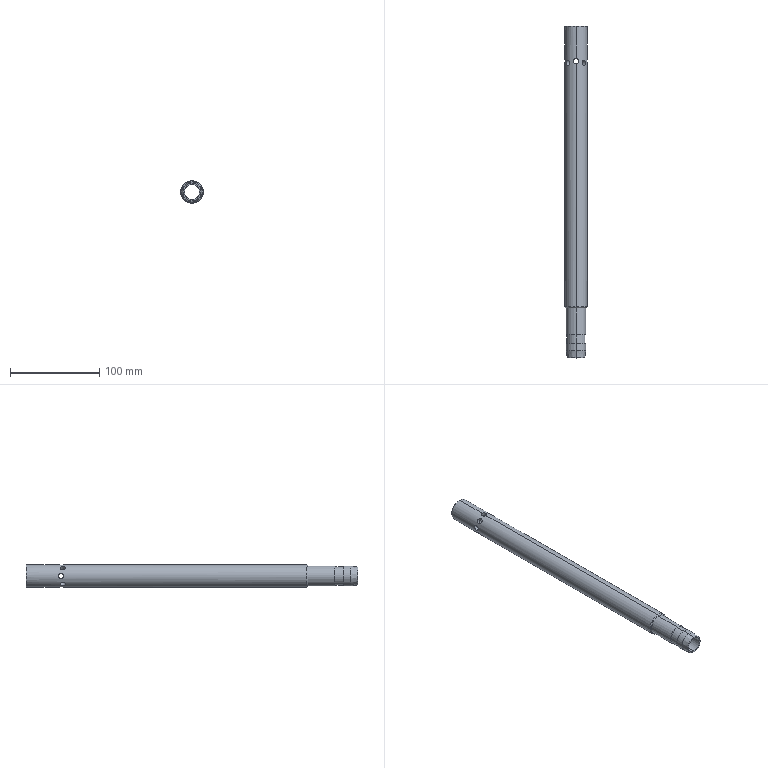Part | SolidWorks | features Chamfer 3, ICE 3, CirPattern 2, Extrusion 1, RefAxis 1, RevCut 1 | 1 solid | 37 faces | box 25 x 371 x 25 mm | volume 90004 mm3 | cylinder 26 | cone 6 | plane 5 | commonest cylinder face diameters 6 x16 22 x4 17 x2 20.6 x2 25 x2